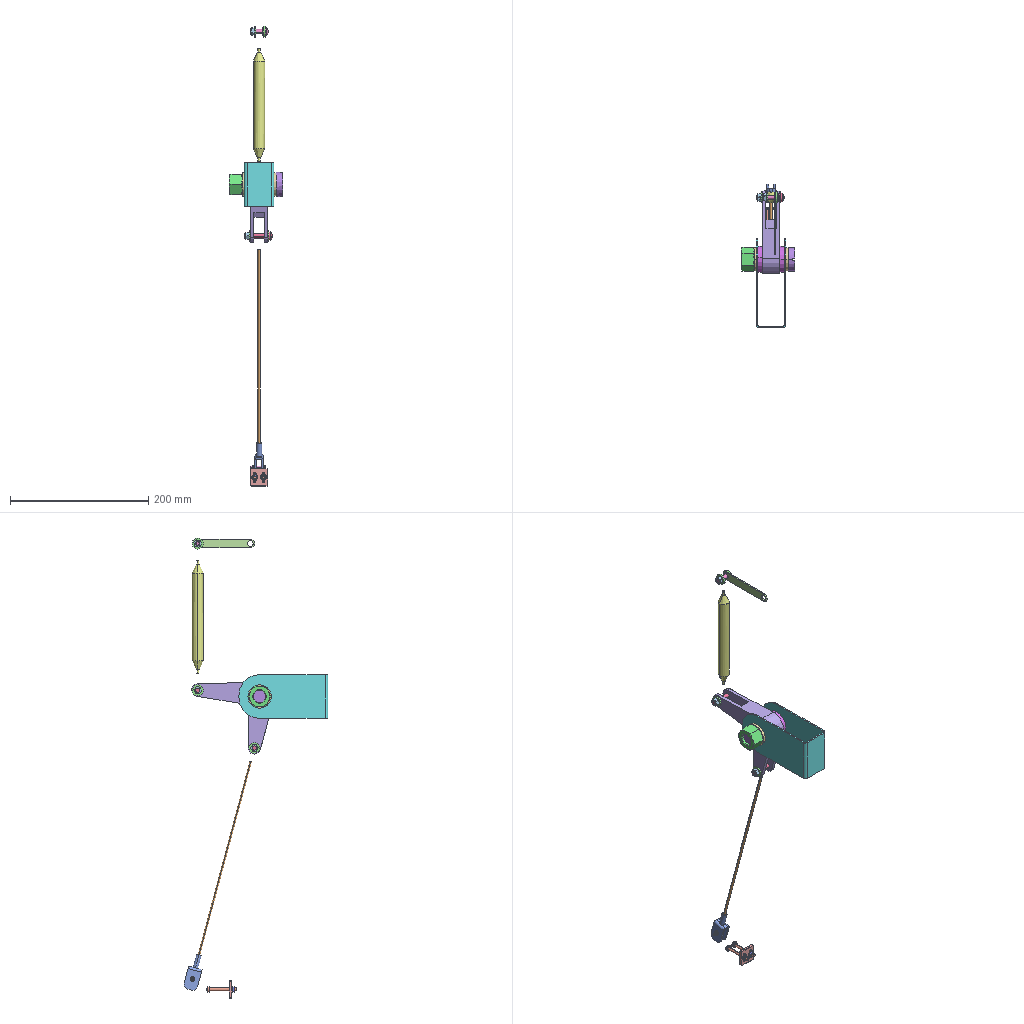Assembly | SolidWorks | 18 different items | 41 placed | box 78 x 208 x 666 mm
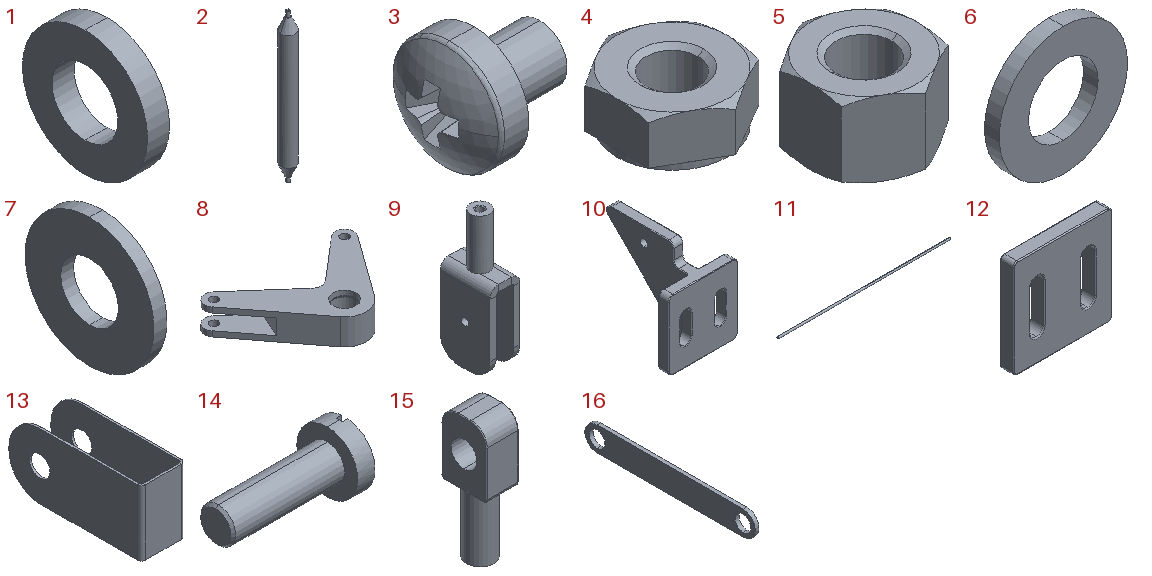Parts list (item | name | quantity | size | volume | features):
1 | - | x2 | 6.7 x 38 x 38 mm | 5494 mm3 | features Extrusion 1
2 | - | x1 | 16.35 x 16.35 x 164.4 mm | 13178 mm3 | features MirrorPattern 2, StudWizard 2, Blend 1, Extrusion 1, ICE 1
3 | - | x6 | 5.046 x 5 x 5 mm | 44.537 mm3 | features RevCut 2, BlendCut 1, CirPattern 1, Fillet 1, LPattern 1, Revolution 1
4 | - | x6 | 7 x 8.083 x 3.2 mm | 105.415 mm3 | features RevCut 4, Extrusion 1, LPattern 1
5 | - | x1 | 8 x 9.238 x 5.6 mm | 229.964 mm3 | features RevCut 3, Extrusion 1, LPattern 1
6 | - | x6 | 14 x 1.6 x 14 mm | 173.718 mm3 | features Revolution 1
7 | - | x8 | 1.6 x 16 x 16 mm | 257.457 mm3 | features Extrusion 1
8 | - | x1 | 134.673 x 93.64 x 25.4 mm | 86753 mm3 | features ICE 6, Extrusion 1, Fillet 1
9 | - | x1 | 12 x 20 x 52.5 mm | 4162 mm3 | features Cut 1, Fillet 1, FlatPattern 1, HoleWzd 1, ICE 1, SMBaseFlange 1, SheetMetal 1
10 | - | x1 | 24.99 x 33.176 x 32.13 mm | 3593 mm3 | features ICE 4, Fillet 3, Extrusion 1, Scale 1
11 | - | x1 | 300 x 3.5 x 3.5 mm | 2885 mm3 | features StudWizard 2, Extrusion 1
12 | - | x1 | 25 x 3.5 x 25 mm | 1868 mm3 | features Extrusion 1, Fillet 1
13 | - | x1 | 42.8 x 129 x 63.5 mm | 34565 mm3 | features Fillet 1, FlatPattern 1, ICE 1, SMBaseFlange 1, SheetMetal 1
14 | - | x1 | 74 x 35 x 35 mm | 29304 mm3 | features ICE 3, Extrusion 1, StudWizard 1
15 | - | x1 | 10 x 14 x 40.005 mm | 3250 mm3 | features Cut 1, Extrusion 1, Fillet 1, HoleWzd 1, ICE 1
16 | - | x1 | 2 x 88.9 x 12.7 mm | 1978 mm3 | features Extrusion 1
17 | XXXXXXXXXXXXXXXXXXXF8DJH | x1 | - | - | -
18 | XXXXXXXXXUVL57 | x1 | - | - | -
Mates (type | each side: item.copy, entity, surface, feature):
Concentric | 9.1 face cylinder Cut-Extrude1 | 7.1 face cylinder Base-Extrude
Coincident | 9.1 face plane Base-Flange1 | 7.1 face plane Base-Extrude
Concentric | 9.1 face cylinder Cut-Extrude1 | 7.2 face cylinder Base-Extrude
Coincident | 9.1 face plane Base-Flange1 | 7.2 face plane Base-Extrude
Concentric | 9.1 face cylinder Cut-Extrude1 | 3.1 face cylinder BaseBody
Coincident | 7.1 face plane Base-Extrude | 3.1 face plane BaseBody
Concentric | 3.1 face cylinder BaseBody | 4.1 face cylinder EndChamfer
Coincident | 7.2 face plane Base-Extrude | 4.1 face plane BaseNut
Concentric | 9.1 face cylinder M3.5 Tapped Hole2 | 11.1 face cylinder Boss-Extrude1
Coincident | 9.1 edge | 11.1 face plane Boss-Extrude1
Concentric | 8.1 face cylinder Boss-Extrude1 | 7.3 face cylinder Base-Extrude
Coincident | 8.1 face plane Boss-Extrude1 | 7.3 face plane Base-Extrude
Concentric | 8.1 face cylinder Boss-Extrude1 | 7.4 face cylinder Base-Extrude
Coincident | 8.1 face plane Boss-Extrude1 | 7.4 face plane Base-Extrude
Concentric | 8.1 face cylinder Boss-Extrude1 | 3.2 face cylinder BaseBody
Coincident | 7.4 face plane Base-Extrude | 3.2 face plane BaseBody
Concentric | 3.2 face cylinder BaseBody | 4.2 face cylinder EndChamfer
Coincident | 7.3 face plane Base-Extrude | 4.2 face plane BaseNut
Concentric | 8.1 face cylinder Boss-Extrude1 | 7.5 face cylinder Base-Extrude
Coincident | 8.1 face plane Boss-Extrude1 | 7.5 face plane Base-Extrude
Concentric | 8.1 face cylinder Boss-Extrude1 | 7.6 face cylinder Base-Extrude
Coincident | 8.1 face plane Boss-Extrude1 | 7.6 face plane Base-Extrude
Concentric | 8.1 face cylinder Boss-Extrude1 | 3.3 face cylinder BaseBody
Coincident | 7.5 face plane Base-Extrude | 3.3 face plane BaseBody
Concentric | 3.3 face cylinder BaseBody | 4.3 face cylinder EndChamfer
Coincident | 7.6 face plane Base-Extrude | 4.3 face plane BaseNut
Concentric | 8.1 face cylinder Boss-Extrude1 | 1.1 face cylinder Boss-Extrude1
Coincident | 8.1 face plane Boss-Extrude1 | 1.1 edge
Concentric | 8.1 face cylinder Boss-Extrude1 | 1.2 face cylinder Boss-Extrude1
Coincident | 8.1 face plane Boss-Extrude1 | 1.2 edge
Width | 12.1 face plane Boss-Extrude1 | 12.1 face plane Boss-Extrude1 | 6.1 face cylinder BaseBody | 2 times
Coincident | 12.1 face plane Boss-Extrude1 | 6.1 face plane BaseBody
Width | 12.1 face plane Boss-Extrude1 | 12.1 face plane Boss-Extrude1 | 6.2 face cylinder BaseBody | 2 times
Coincident | 12.1 face plane Boss-Extrude1 | 6.2 face plane BaseBody
Concentric | 6.3 face cylinder BaseBody | 3.4 face cylinder BaseBody
Coincident | 6.3 face plane BaseBody | 3.4 face plane BaseBody
Concentric | 6.4 face cylinder BaseBody | 3.5 face cylinder BaseBody
Coincident | 6.4 face plane BaseBody | 3.5 face plane BaseBody
Concentric | 3.4 face cylinder BaseBody | 4.4 face cylinder EndChamfer
Concentric | 3.5 face cylinder BaseBody | 4.5 face cylinder EndChamfer
Coincident | 6.1 face plane BaseBody | 4.4 face plane BaseNut
Coincident | 6.2 face plane BaseBody | 4.5 face plane BaseNut
Concentric | 16.1 face cylinder Boss-Extrude1 | 7.7 face cylinder Base-Extrude
Coincident | 16.1 face plane Boss-Extrude1 | 7.7 face plane Base-Extrude
Concentric | 7.7 face cylinder Base-Extrude | 3.6 face cylinder BaseBody
Coincident | 7.7 face plane Base-Extrude | 3.6 face plane BaseBody
Concentric | 3.6 face cylinder BaseBody | 4.6 face cylinder EndChamfer
Coincident | 7.8 face plane Base-Extrude | 4.6 face plane BaseNut
Width | 1.2 face plane Boss-Extrude1 | 1.1 face plane Boss-Extrude1 | 13.1 face plane Base-Flange1 | 13.1 face plane Base-Flange1
Concentric | 1.1 face cylinder Boss-Extrude1 | 13.1 face cylinder Cut-Extrude1
Parallel | 12.1 face plane Boss-Extrude1 | 13.1 face plane Base-Flange1
Concentric | 13.1 face cylinder Cut-Extrude1 | 6.5 face cylinder BaseBody
Coincident | 13.1 face plane Base-Flange1 | 6.5 face plane BaseBody
Coincident | 13.1 face plane Base-Flange1 | 6.6 face plane BaseBody
Concentric | 13.1 face cylinder Cut-Extrude1 | 6.6 face cylinder BaseBody
Concentric | 6.6 face cylinder BaseBody | 14.1 face cylinder Boss-Extrude2
Coincident | 6.6 face plane BaseBody | 14.1 face plane Boss-Extrude1
Parallel | 13.1 face plane Base-Flange1 | 14.1 face plane Cut-Extrude1
Concentric | 14.1 face cone M20 Machine Threads Stud1 | 5.1 face cylinder EndChamfer
Coincident | 6.5 face plane BaseBody | 5.1 face plane BaseNut